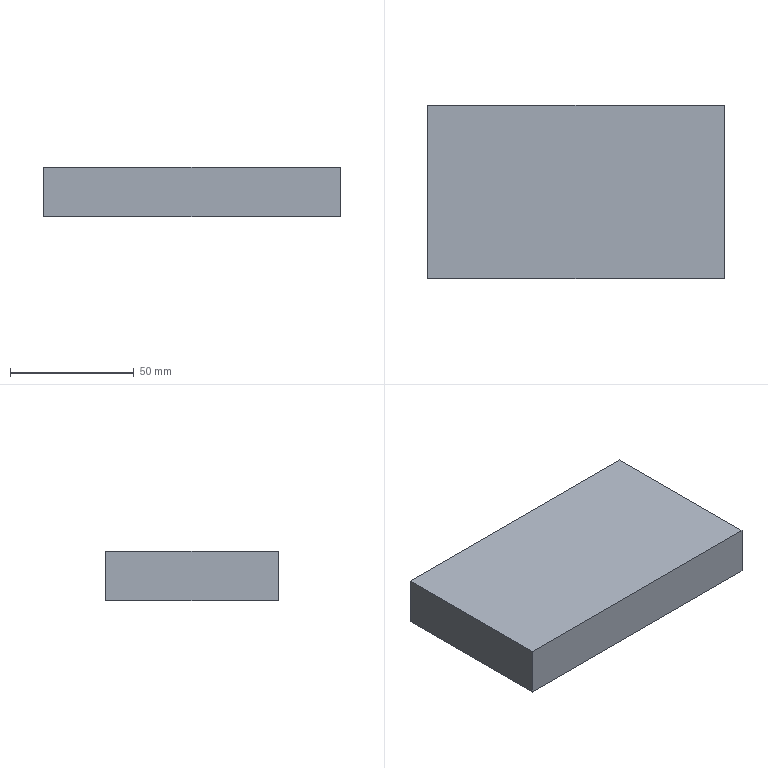Part | STEP file | Tube necking machine_id562_x_t | 1 solid | 6 faces | box 120 x 70 x 20 mm | volume 168000 mm3 | plane 6
STEP:
#1=CARTESIAN_POINT('',(0.,0.,0.));
#2=DIRECTION('',(0.,0.,1.));
#3=DIRECTION('',(1.,0.,0.));
#4=AXIS2_PLACEMENT_3D('',#1,#2,#3);
#5=CARTESIAN_POINT('',(210.,85.,0.));
#6=VERTEX_POINT('',#5);
#7=CARTESIAN_POINT('',(210.,15.,0.));
#8=VERTEX_POINT('',#7);
#9=CARTESIAN_POINT('',(210.,85.,0.));
#10=DIRECTION('',(0.,-1.,0.));
#11=VECTOR('',#10,1.);
#12=LINE('',#9,#11);
#13=CARTESIAN_POINT('',(210.,85.,20.));
#14=DIRECTION('',(1.,0.,0.));
#15=DIRECTION('',(0.,0.,-1.));
#16=AXIS2_PLACEMENT_3D('',#13,#14,#15);
#17=PLANE('',#16);
#18=CARTESIAN_POINT('',(20.,0.));
#19=DIRECTION('',(0.,-1.));
#20=VECTOR('',#19,1.);
#21=LINE('',#18,#20);
#22=(GEOMETRIC_REPRESENTATION_CONTEXT(2)PARAMETRIC_REPRESENTATION_CONTEXT()REPRESENTATION_CONTEXT('',''));
#23=DEFINITIONAL_REPRESENTATION('',(#21),#22);
#24=PCURVE('',#17,#23);
#25=CARTESIAN_POINT('',(2.5,0.,0.));
#26=DIRECTION('',(0.,0.,1.));
#27=DIRECTION('',(1.,0.,0.));
#28=AXIS2_PLACEMENT_3D('',#25,#26,#27);
#29=PLANE('',#28);
#30=CARTESIAN_POINT('',(207.5,85.));
#31=DIRECTION('',(0.,-1.));
#32=VECTOR('',#31,1.);
#33=LINE('',#30,#32);
#34=(GEOMETRIC_REPRESENTATION_CONTEXT(2)PARAMETRIC_REPRESENTATION_CONTEXT()REPRESENTATION_CONTEXT('',''));
#35=DEFINITIONAL_REPRESENTATION('',(#33),#34);
#36=PCURVE('',#29,#35);
#37=SURFACE_CURVE('',#12,(#24,#36),.PCURVE_S1.);
#38=EDGE_CURVE('',#6,#8,#37,.T.);
#39=ORIENTED_EDGE('',*,*,#38,.T.);
#40=CARTESIAN_POINT('',(210.,15.,20.));
#41=VERTEX_POINT('',#40);
#42=CARTESIAN_POINT('',(210.,15.,20.));
#43=DIRECTION('',(0.,0.,-1.));
#44=VECTOR('',#43,1.);
#45=LINE('',#42,#44);
#46=CARTESIAN_POINT('',(0.,-70.));
#47=DIRECTION('',(1.,0.));
#48=VECTOR('',#47,1.);
#49=LINE('',#46,#48);
#50=(GEOMETRIC_REPRESENTATION_CONTEXT(2)PARAMETRIC_REPRESENTATION_CONTEXT()REPRESENTATION_CONTEXT('',''));
#51=DEFINITIONAL_REPRESENTATION('',(#49),#50);
#52=PCURVE('',#17,#51);
#53=CARTESIAN_POINT('',(210.,15.,20.));
#54=DIRECTION('',(0.,1.,0.));
#55=DIRECTION('',(0.,0.,1.));
#56=AXIS2_PLACEMENT_3D('',#53,#54,#55);
#57=PLANE('',#56);
#58=CARTESIAN_POINT('',(0.,0.));
#59=DIRECTION('',(-1.,0.));
#60=VECTOR('',#59,1.);
#61=LINE('',#58,#60);
#62=(GEOMETRIC_REPRESENTATION_CONTEXT(2)PARAMETRIC_REPRESENTATION_CONTEXT()REPRESENTATION_CONTEXT('',''));
#63=DEFINITIONAL_REPRESENTATION('',(#61),#62);
#64=PCURVE('',#57,#63);
#65=SURFACE_CURVE('',#45,(#52,#64),.PCURVE_S1.);
#66=EDGE_CURVE('',#41,#8,#65,.T.);
#67=ORIENTED_EDGE('',*,*,#66,.F.);
#68=CARTESIAN_POINT('',(210.,85.,20.));
#69=VERTEX_POINT('',#68);
#70=CARTESIAN_POINT('',(210.,85.,20.));
#71=DIRECTION('',(0.,-1.,0.));
#72=VECTOR('',#71,1.);
#73=LINE('',#70,#72);
#74=CARTESIAN_POINT('',(0.,0.));
#75=DIRECTION('',(0.,-1.));
#76=VECTOR('',#75,1.);
#77=LINE('',#74,#76);
#78=(GEOMETRIC_REPRESENTATION_CONTEXT(2)PARAMETRIC_REPRESENTATION_CONTEXT()REPRESENTATION_CONTEXT('',''));
#79=DEFINITIONAL_REPRESENTATION('',(#77),#78);
#80=PCURVE('',#17,#79);
#81=CARTESIAN_POINT('',(2.5,0.,20.));
#82=DIRECTION('',(0.,0.,1.));
#83=DIRECTION('',(1.,0.,0.));
#84=AXIS2_PLACEMENT_3D('',#81,#82,#83);
#85=PLANE('',#84);
#86=CARTESIAN_POINT('',(207.5,85.));
#87=DIRECTION('',(0.,-1.));
#88=VECTOR('',#87,1.);
#89=LINE('',#86,#88);
#90=(GEOMETRIC_REPRESENTATION_CONTEXT(2)PARAMETRIC_REPRESENTATION_CONTEXT()REPRESENTATION_CONTEXT('',''));
#91=DEFINITIONAL_REPRESENTATION('',(#89),#90);
#92=PCURVE('',#85,#91);
#93=SURFACE_CURVE('',#73,(#80,#92),.PCURVE_S1.);
#94=EDGE_CURVE('',#69,#41,#93,.T.);
#95=ORIENTED_EDGE('',*,*,#94,.F.);
#96=CARTESIAN_POINT('',(210.,85.,20.));
#97=DIRECTION('',(0.,0.,-1.));
#98=VECTOR('',#97,1.);
#99=LINE('',#96,#98);
#100=CARTESIAN_POINT('',(0.,0.));
#101=DIRECTION('',(1.,0.));
#102=VECTOR('',#101,1.);
#103=LINE('',#100,#102);
#104=(GEOMETRIC_REPRESENTATION_CONTEXT(2)PARAMETRIC_REPRESENTATION_CONTEXT()REPRESENTATION_CONTEXT('',''));
#105=DEFINITIONAL_REPRESENTATION('',(#103),#104);
#106=PCURVE('',#17,#105);
#107=CARTESIAN_POINT('',(330.,85.,20.));
#108=DIRECTION('',(0.,-1.,0.));
#109=DIRECTION('',(0.,0.,-1.));
#110=AXIS2_PLACEMENT_3D('',#107,#108,#109);
#111=PLANE('',#110);
#112=CARTESIAN_POINT('',(0.,-120.));
#113=DIRECTION('',(1.,0.));
#114=VECTOR('',#113,1.);
#115=LINE('',#112,#114);
#116=(GEOMETRIC_REPRESENTATION_CONTEXT(2)PARAMETRIC_REPRESENTATION_CONTEXT()REPRESENTATION_CONTEXT('',''));
#117=DEFINITIONAL_REPRESENTATION('',(#115),#116);
#118=PCURVE('',#111,#117);
#119=SURFACE_CURVE('',#99,(#106,#118),.PCURVE_S1.);
#120=EDGE_CURVE('',#69,#6,#119,.T.);
#121=ORIENTED_EDGE('',*,*,#120,.T.);
#122=EDGE_LOOP('',(#39,#67,#95,#121));
#123=FACE_BOUND('',#122,.T.);
#124=ADVANCED_FACE('',(#123),#17,.F.);
#125=CARTESIAN_POINT('',(330.,15.,0.));
#126=VERTEX_POINT('',#125);
#127=CARTESIAN_POINT('',(210.,15.,0.));
#128=DIRECTION('',(1.,0.,0.));
#129=VECTOR('',#128,1.);
#130=LINE('',#127,#129);
#131=CARTESIAN_POINT('',(-20.,0.));
#132=DIRECTION('',(0.,1.));
#133=VECTOR('',#132,1.);
#134=LINE('',#131,#133);
#135=(GEOMETRIC_REPRESENTATION_CONTEXT(2)PARAMETRIC_REPRESENTATION_CONTEXT()REPRESENTATION_CONTEXT('',''));
#136=DEFINITIONAL_REPRESENTATION('',(#134),#135);
#137=PCURVE('',#57,#136);
#138=CARTESIAN_POINT('',(207.5,15.));
#139=DIRECTION('',(1.,0.));
#140=VECTOR('',#139,1.);
#141=LINE('',#138,#140);
#142=(GEOMETRIC_REPRESENTATION_CONTEXT(2)PARAMETRIC_REPRESENTATION_CONTEXT()REPRESENTATION_CONTEXT('',''));
#143=DEFINITIONAL_REPRESENTATION('',(#141),#142);
#144=PCURVE('',#29,#143);
#145=SURFACE_CURVE('',#130,(#137,#144),.PCURVE_S1.);
#146=EDGE_CURVE('',#8,#126,#145,.T.);
#147=ORIENTED_EDGE('',*,*,#146,.T.);
#148=CARTESIAN_POINT('',(330.,15.,20.));
#149=VERTEX_POINT('',#148);
#150=CARTESIAN_POINT('',(330.,15.,20.));
#151=DIRECTION('',(0.,0.,-1.));
#152=VECTOR('',#151,1.);
#153=LINE('',#150,#152);
#154=CARTESIAN_POINT('',(0.,120.));
#155=DIRECTION('',(-1.,0.));
#156=VECTOR('',#155,1.);
#157=LINE('',#154,#156);
#158=(GEOMETRIC_REPRESENTATION_CONTEXT(2)PARAMETRIC_REPRESENTATION_CONTEXT()REPRESENTATION_CONTEXT('',''));
#159=DEFINITIONAL_REPRESENTATION('',(#157),#158);
#160=PCURVE('',#57,#159);
#161=CARTESIAN_POINT('',(330.,15.,20.));
#162=DIRECTION('',(-1.,0.,0.));
#163=DIRECTION('',(0.,0.,1.));
#164=AXIS2_PLACEMENT_3D('',#161,#162,#163);
#165=PLANE('',#164);
#166=CARTESIAN_POINT('',(0.,0.));
#167=DIRECTION('',(-1.,0.));
#168=VECTOR('',#167,1.);
#169=LINE('',#166,#168);
#170=(GEOMETRIC_REPRESENTATION_CONTEXT(2)PARAMETRIC_REPRESENTATION_CONTEXT()REPRESENTATION_CONTEXT('',''));
#171=DEFINITIONAL_REPRESENTATION('',(#169),#170);
#172=PCURVE('',#165,#171);
#173=SURFACE_CURVE('',#153,(#160,#172),.PCURVE_S1.);
#174=EDGE_CURVE('',#149,#126,#173,.T.);
#175=ORIENTED_EDGE('',*,*,#174,.F.);
#176=CARTESIAN_POINT('',(210.,15.,20.));
#177=DIRECTION('',(1.,0.,0.));
#178=VECTOR('',#177,1.);
#179=LINE('',#176,#178);
#180=CARTESIAN_POINT('',(0.,0.));
#181=DIRECTION('',(0.,1.));
#182=VECTOR('',#181,1.);
#183=LINE('',#180,#182);
#184=(GEOMETRIC_REPRESENTATION_CONTEXT(2)PARAMETRIC_REPRESENTATION_CONTEXT()REPRESENTATION_CONTEXT('',''));
#185=DEFINITIONAL_REPRESENTATION('',(#183),#184);
#186=PCURVE('',#57,#185);
#187=CARTESIAN_POINT('',(207.5,15.));
#188=DIRECTION('',(1.,0.));
#189=VECTOR('',#188,1.);
#190=LINE('',#187,#189);
#191=(GEOMETRIC_REPRESENTATION_CONTEXT(2)PARAMETRIC_REPRESENTATION_CONTEXT()REPRESENTATION_CONTEXT('',''));
#192=DEFINITIONAL_REPRESENTATION('',(#190),#191);
#193=PCURVE('',#85,#192);
#194=SURFACE_CURVE('',#179,(#186,#193),.PCURVE_S1.);
#195=EDGE_CURVE('',#41,#149,#194,.T.);
#196=ORIENTED_EDGE('',*,*,#195,.F.);
#197=ORIENTED_EDGE('',*,*,#66,.T.);
#198=EDGE_LOOP('',(#147,#175,#196,#197));
#199=FACE_BOUND('',#198,.T.);
#200=ADVANCED_FACE('',(#199),#57,.F.);
#201=CARTESIAN_POINT('',(330.,85.,0.));
#202=VERTEX_POINT('',#201);
#203=CARTESIAN_POINT('',(330.,15.,0.));
#204=DIRECTION('',(0.,1.,0.));
#205=VECTOR('',#204,1.);
#206=LINE('',#203,#205);
#207=CARTESIAN_POINT('',(-20.,0.));
#208=DIRECTION('',(0.,1.));
#209=VECTOR('',#208,1.);
#210=LINE('',#207,#209);
#211=(GEOMETRIC_REPRESENTATION_CONTEXT(2)PARAMETRIC_REPRESENTATION_CONTEXT()REPRESENTATION_CONTEXT('',''));
#212=DEFINITIONAL_REPRESENTATION('',(#210),#211);
#213=PCURVE('',#165,#212);
#214=CARTESIAN_POINT('',(327.5,15.));
#215=DIRECTION('',(0.,1.));
#216=VECTOR('',#215,1.);
#217=LINE('',#214,#216);
#218=(GEOMETRIC_REPRESENTATION_CONTEXT(2)PARAMETRIC_REPRESENTATION_CONTEXT()REPRESENTATION_CONTEXT('',''));
#219=DEFINITIONAL_REPRESENTATION('',(#217),#218);
#220=PCURVE('',#29,#219);
#221=SURFACE_CURVE('',#206,(#213,#220),.PCURVE_S1.);
#222=EDGE_CURVE('',#126,#202,#221,.T.);
#223=ORIENTED_EDGE('',*,*,#222,.T.);
#224=CARTESIAN_POINT('',(330.,85.,20.));
#225=VERTEX_POINT('',#224);
#226=CARTESIAN_POINT('',(330.,85.,20.));
#227=DIRECTION('',(0.,0.,-1.));
#228=VECTOR('',#227,1.);
#229=LINE('',#226,#228);
#230=CARTESIAN_POINT('',(0.,70.));
#231=DIRECTION('',(-1.,0.));
#232=VECTOR('',#231,1.);
#233=LINE('',#230,#232);
#234=(GEOMETRIC_REPRESENTATION_CONTEXT(2)PARAMETRIC_REPRESENTATION_CONTEXT()REPRESENTATION_CONTEXT('',''));
#235=DEFINITIONAL_REPRESENTATION('',(#233),#234);
#236=PCURVE('',#165,#235);
#237=CARTESIAN_POINT('',(0.,0.));
#238=DIRECTION('',(1.,0.));
#239=VECTOR('',#238,1.);
#240=LINE('',#237,#239);
#241=(GEOMETRIC_REPRESENTATION_CONTEXT(2)PARAMETRIC_REPRESENTATION_CONTEXT()REPRESENTATION_CONTEXT('',''));
#242=DEFINITIONAL_REPRESENTATION('',(#240),#241);
#243=PCURVE('',#111,#242);
#244=SURFACE_CURVE('',#229,(#236,#243),.PCURVE_S1.);
#245=EDGE_CURVE('',#225,#202,#244,.T.);
#246=ORIENTED_EDGE('',*,*,#245,.F.);
#247=CARTESIAN_POINT('',(330.,15.,20.));
#248=DIRECTION('',(0.,1.,0.));
#249=VECTOR('',#248,1.);
#250=LINE('',#247,#249);
#251=CARTESIAN_POINT('',(0.,0.));
#252=DIRECTION('',(0.,1.));
#253=VECTOR('',#252,1.);
#254=LINE('',#251,#253);
#255=(GEOMETRIC_REPRESENTATION_CONTEXT(2)PARAMETRIC_REPRESENTATION_CONTEXT()REPRESENTATION_CONTEXT('',''));
#256=DEFINITIONAL_REPRESENTATION('',(#254),#255);
#257=PCURVE('',#165,#256);
#258=CARTESIAN_POINT('',(327.5,15.));
#259=DIRECTION('',(0.,1.));
#260=VECTOR('',#259,1.);
#261=LINE('',#258,#260);
#262=(GEOMETRIC_REPRESENTATION_CONTEXT(2)PARAMETRIC_REPRESENTATION_CONTEXT()REPRESENTATION_CONTEXT('',''));
#263=DEFINITIONAL_REPRESENTATION('',(#261),#262);
#264=PCURVE('',#85,#263);
#265=SURFACE_CURVE('',#250,(#257,#264),.PCURVE_S1.);
#266=EDGE_CURVE('',#149,#225,#265,.T.);
#267=ORIENTED_EDGE('',*,*,#266,.F.);
#268=ORIENTED_EDGE('',*,*,#174,.T.);
#269=EDGE_LOOP('',(#223,#246,#267,#268));
#270=FACE_BOUND('',#269,.T.);
#271=ADVANCED_FACE('',(#270),#165,.F.);
#272=CARTESIAN_POINT('',(330.,85.,0.));
#273=DIRECTION('',(-1.,0.,0.));
#274=VECTOR('',#273,1.);
#275=LINE('',#272,#274);
#276=CARTESIAN_POINT('',(20.,0.));
#277=DIRECTION('',(0.,-1.));
#278=VECTOR('',#277,1.);
#279=LINE('',#276,#278);
#280=(GEOMETRIC_REPRESENTATION_CONTEXT(2)PARAMETRIC_REPRESENTATION_CONTEXT()REPRESENTATION_CONTEXT('',''));
#281=DEFINITIONAL_REPRESENTATION('',(#279),#280);
#282=PCURVE('',#111,#281);
#283=CARTESIAN_POINT('',(327.5,85.));
#284=DIRECTION('',(-1.,0.));
#285=VECTOR('',#284,1.);
#286=LINE('',#283,#285);
#287=(GEOMETRIC_REPRESENTATION_CONTEXT(2)PARAMETRIC_REPRESENTATION_CONTEXT()REPRESENTATION_CONTEXT('',''));
#288=DEFINITIONAL_REPRESENTATION('',(#286),#287);
#289=PCURVE('',#29,#288);
#290=SURFACE_CURVE('',#275,(#282,#289),.PCURVE_S1.);
#291=EDGE_CURVE('',#202,#6,#290,.T.);
#292=ORIENTED_EDGE('',*,*,#291,.T.);
#293=ORIENTED_EDGE('',*,*,#120,.F.);
#294=CARTESIAN_POINT('',(330.,85.,20.));
#295=DIRECTION('',(-1.,0.,0.));
#296=VECTOR('',#295,1.);
#297=LINE('',#294,#296);
#298=CARTESIAN_POINT('',(0.,0.));
#299=DIRECTION('',(0.,-1.));
#300=VECTOR('',#299,1.);
#301=LINE('',#298,#300);
#302=(GEOMETRIC_REPRESENTATION_CONTEXT(2)PARAMETRIC_REPRESENTATION_CONTEXT()REPRESENTATION_CONTEXT('',''));
#303=DEFINITIONAL_REPRESENTATION('',(#301),#302);
#304=PCURVE('',#111,#303);
#305=CARTESIAN_POINT('',(327.5,85.));
#306=DIRECTION('',(-1.,0.));
#307=VECTOR('',#306,1.);
#308=LINE('',#305,#307);
#309=(GEOMETRIC_REPRESENTATION_CONTEXT(2)PARAMETRIC_REPRESENTATION_CONTEXT()REPRESENTATION_CONTEXT('',''));
#310=DEFINITIONAL_REPRESENTATION('',(#308),#309);
#311=PCURVE('',#85,#310);
#312=SURFACE_CURVE('',#297,(#304,#311),.PCURVE_S1.);
#313=EDGE_CURVE('',#225,#69,#312,.T.);
#314=ORIENTED_EDGE('',*,*,#313,.F.);
#315=ORIENTED_EDGE('',*,*,#245,.T.);
#316=EDGE_LOOP('',(#292,#293,#314,#315));
#317=FACE_BOUND('',#316,.T.);
#318=ADVANCED_FACE('',(#317),#111,.F.);
#319=ORIENTED_EDGE('',*,*,#94,.T.);
#320=ORIENTED_EDGE('',*,*,#195,.T.);
#321=ORIENTED_EDGE('',*,*,#266,.T.);
#322=ORIENTED_EDGE('',*,*,#313,.T.);
#323=EDGE_LOOP('',(#319,#320,#321,#322));
#324=FACE_BOUND('',#323,.T.);
#325=ADVANCED_FACE('',(#324),#85,.T.);
#326=ORIENTED_EDGE('',*,*,#38,.F.);
#327=ORIENTED_EDGE('',*,*,#291,.F.);
#328=ORIENTED_EDGE('',*,*,#222,.F.);
#329=ORIENTED_EDGE('',*,*,#146,.F.);
#330=EDGE_LOOP('',(#326,#327,#328,#329));
#331=FACE_BOUND('',#330,.T.);
#332=ADVANCED_FACE('',(#331),#29,.F.);
#333=CLOSED_SHELL('',(#124,#200,#271,#318,#325,#332));
#334=MANIFOLD_SOLID_BREP('',#333);
#335=(LENGTH_UNIT()NAMED_UNIT(*)SI_UNIT(.MILLI.,.METRE.));
#336=UNCERTAINTY_MEASURE_WITH_UNIT(LENGTH_MEASURE(0.0000001),#335,'','');
#337=(NAMED_UNIT(*)PLANE_ANGLE_UNIT()SI_UNIT($,.RADIAN.));
#338=(NAMED_UNIT(*)SI_UNIT($,.STERADIAN.)SOLID_ANGLE_UNIT());
#339=(GEOMETRIC_REPRESENTATION_CONTEXT(3)GLOBAL_UNCERTAINTY_ASSIGNED_CONTEXT((#336))GLOBAL_UNIT_ASSIGNED_CONTEXT((#335,#337,#338))REPRESENTATION_CONTEXT('',''));
#340=ADVANCED_BREP_SHAPE_REPRESENTATION('',(#4,#334),#339);